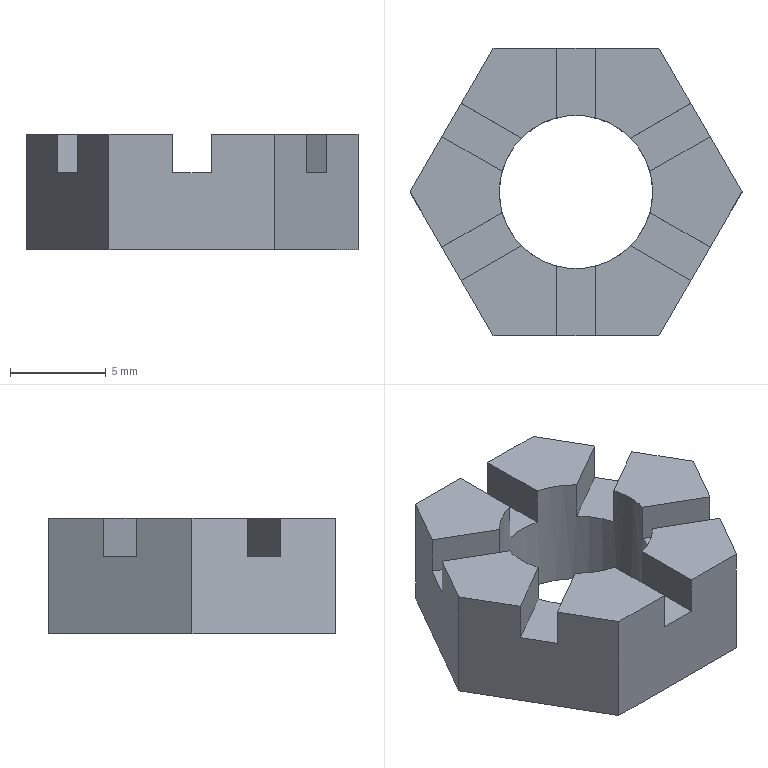Part | SolidWorks | features BaseBody 1 | 1 solid | 33 faces | box 17.321 x 15 x 6 mm | volume 782.532 mm3 | plane 31 | cylinder 2 | commonest cylinder face diameters 8 x2
STEP:
#1=CARTESIAN_POINT('',(4.,0.,6.));
#2=VERTEX_POINT('',#1);
#3=CARTESIAN_POINT('',(3.854,-1.07,6.));
#4=VERTEX_POINT('',#3);
#5=CARTESIAN_POINT('',(0.,0.,6.));
#6=DIRECTION('',(0.,0.,-1.));
#7=DIRECTION('',(-1.,0.,0.));
#8=AXIS2_PLACEMENT_3D('',#5,#6,#7);
#9=CIRCLE('',#8,4.);
#10=EDGE_CURVE('',#2,#4,#9,.T.);
#11=ORIENTED_EDGE('',*,*,#10,.F.);
#12=CARTESIAN_POINT('',(4.,0.,0.));
#13=VERTEX_POINT('',#12);
#14=CARTESIAN_POINT('',(4.,0.,0.));
#15=DIRECTION('',(0.,0.,-1.));
#16=VECTOR('',#15,1000.);
#17=LINE('',#14,#16);
#18=EDGE_CURVE('',#2,#13,#17,.T.);
#19=ORIENTED_EDGE('',*,*,#18,.T.);
#20=CARTESIAN_POINT('',(-4.,0.,0.));
#21=VERTEX_POINT('',#20);
#22=CARTESIAN_POINT('',(0.,0.,0.));
#23=DIRECTION('',(0.,0.,1.));
#24=DIRECTION('',(-1.,0.,0.));
#25=AXIS2_PLACEMENT_3D('',#22,#23,#24);
#26=CIRCLE('',#25,4.);
#27=EDGE_CURVE('',#21,#13,#26,.T.);
#28=ORIENTED_EDGE('',*,*,#27,.F.);
#29=CARTESIAN_POINT('',(-4.,0.,6.));
#30=VERTEX_POINT('',#29);
#31=CARTESIAN_POINT('',(-4.,0.,0.));
#32=DIRECTION('',(0.,0.,-1.));
#33=VECTOR('',#32,1000.);
#34=LINE('',#31,#33);
#35=EDGE_CURVE('',#30,#21,#34,.T.);
#36=ORIENTED_EDGE('',*,*,#35,.F.);
#37=CARTESIAN_POINT('',(-3.854,-1.07,6.));
#38=VERTEX_POINT('',#37);
#39=CARTESIAN_POINT('',(0.,0.,6.));
#40=DIRECTION('',(0.,0.,-1.));
#41=DIRECTION('',(-1.,0.,0.));
#42=AXIS2_PLACEMENT_3D('',#39,#40,#41);
#43=CIRCLE('',#42,4.);
#44=EDGE_CURVE('',#38,#30,#43,.T.);
#45=ORIENTED_EDGE('',*,*,#44,.F.);
#46=CARTESIAN_POINT('',(-3.854,-1.07,4.));
#47=VERTEX_POINT('',#46);
#48=CARTESIAN_POINT('',(-3.854,-1.07,0.));
#49=DIRECTION('',(0.,0.,-1.));
#50=VECTOR('',#49,1000.);
#51=LINE('',#48,#50);
#52=EDGE_CURVE('',#38,#47,#51,.T.);
#53=ORIENTED_EDGE('',*,*,#52,.T.);
#54=CARTESIAN_POINT('',(-2.854,-2.803,4.));
#55=VERTEX_POINT('',#54);
#56=CARTESIAN_POINT('',(0.,0.,4.));
#57=DIRECTION('',(0.,0.,1.));
#58=DIRECTION('',(-1.,0.,0.));
#59=AXIS2_PLACEMENT_3D('',#56,#57,#58);
#60=CIRCLE('',#59,4.);
#61=EDGE_CURVE('',#47,#55,#60,.T.);
#62=ORIENTED_EDGE('',*,*,#61,.T.);
#63=CARTESIAN_POINT('',(-2.854,-2.803,6.));
#64=VERTEX_POINT('',#63);
#65=CARTESIAN_POINT('',(-2.854,-2.803,0.));
#66=DIRECTION('',(0.,0.,1.));
#67=VECTOR('',#66,1000.);
#68=LINE('',#65,#67);
#69=EDGE_CURVE('',#55,#64,#68,.T.);
#70=ORIENTED_EDGE('',*,*,#69,.T.);
#71=CARTESIAN_POINT('',(-1.,-3.873,6.));
#72=VERTEX_POINT('',#71);
#73=CARTESIAN_POINT('',(0.,0.,6.));
#74=DIRECTION('',(0.,0.,-1.));
#75=DIRECTION('',(-1.,0.,0.));
#76=AXIS2_PLACEMENT_3D('',#73,#74,#75);
#77=CIRCLE('',#76,4.);
#78=EDGE_CURVE('',#72,#64,#77,.T.);
#79=ORIENTED_EDGE('',*,*,#78,.F.);
#80=CARTESIAN_POINT('',(-1.,-3.873,4.));
#81=VERTEX_POINT('',#80);
#82=CARTESIAN_POINT('',(-1.,-3.873,0.));
#83=DIRECTION('',(0.,0.,-1.));
#84=VECTOR('',#83,1000.);
#85=LINE('',#82,#84);
#86=EDGE_CURVE('',#72,#81,#85,.T.);
#87=ORIENTED_EDGE('',*,*,#86,.T.);
#88=CARTESIAN_POINT('',(1.,-3.873,4.));
#89=VERTEX_POINT('',#88);
#90=CARTESIAN_POINT('',(0.,0.,4.));
#91=DIRECTION('',(0.,0.,1.));
#92=DIRECTION('',(-1.,0.,0.));
#93=AXIS2_PLACEMENT_3D('',#90,#91,#92);
#94=CIRCLE('',#93,4.);
#95=EDGE_CURVE('',#81,#89,#94,.T.);
#96=ORIENTED_EDGE('',*,*,#95,.T.);
#97=CARTESIAN_POINT('',(1.,-3.873,6.));
#98=VERTEX_POINT('',#97);
#99=CARTESIAN_POINT('',(1.,-3.873,0.));
#100=DIRECTION('',(0.,0.,1.));
#101=VECTOR('',#100,1000.);
#102=LINE('',#99,#101);
#103=EDGE_CURVE('',#89,#98,#102,.T.);
#104=ORIENTED_EDGE('',*,*,#103,.T.);
#105=CARTESIAN_POINT('',(2.854,-2.803,6.));
#106=VERTEX_POINT('',#105);
#107=CARTESIAN_POINT('',(0.,0.,6.));
#108=DIRECTION('',(0.,0.,-1.));
#109=DIRECTION('',(-1.,0.,0.));
#110=AXIS2_PLACEMENT_3D('',#107,#108,#109);
#111=CIRCLE('',#110,4.);
#112=EDGE_CURVE('',#106,#98,#111,.T.);
#113=ORIENTED_EDGE('',*,*,#112,.F.);
#114=CARTESIAN_POINT('',(2.854,-2.803,4.));
#115=VERTEX_POINT('',#114);
#116=CARTESIAN_POINT('',(2.854,-2.803,0.));
#117=DIRECTION('',(0.,0.,-1.));
#118=VECTOR('',#117,1000.);
#119=LINE('',#116,#118);
#120=EDGE_CURVE('',#106,#115,#119,.T.);
#121=ORIENTED_EDGE('',*,*,#120,.T.);
#122=CARTESIAN_POINT('',(3.854,-1.07,4.));
#123=VERTEX_POINT('',#122);
#124=CARTESIAN_POINT('',(0.,0.,4.));
#125=DIRECTION('',(0.,0.,1.));
#126=DIRECTION('',(-1.,0.,0.));
#127=AXIS2_PLACEMENT_3D('',#124,#125,#126);
#128=CIRCLE('',#127,4.);
#129=EDGE_CURVE('',#115,#123,#128,.T.);
#130=ORIENTED_EDGE('',*,*,#129,.T.);
#131=CARTESIAN_POINT('',(3.854,-1.07,0.));
#132=DIRECTION('',(0.,0.,1.));
#133=VECTOR('',#132,1000.);
#134=LINE('',#131,#133);
#135=EDGE_CURVE('',#123,#4,#134,.T.);
#136=ORIENTED_EDGE('',*,*,#135,.T.);
#137=EDGE_LOOP('',(#11,#19,#28,#36,#45,#53,#62,#70,#79,#87,#96,#104,#113,#121,#130,#136));
#138=FACE_OUTER_BOUND('',#137,.T.);
#139=CARTESIAN_POINT('',(0.,0.,0.));
#140=DIRECTION('',(0.,0.,-1.));
#141=DIRECTION('',(-1.,0.,0.));
#142=AXIS2_PLACEMENT_3D('',#139,#140,#141);
#143=CYLINDRICAL_SURFACE('',#142,4.);
#144=ADVANCED_FACE('',(#138),#143,.F.);
#145=CARTESIAN_POINT('',(-3.854,1.07,4.));
#146=VERTEX_POINT('',#145);
#147=CARTESIAN_POINT('',(-3.854,1.07,6.));
#148=VERTEX_POINT('',#147);
#149=CARTESIAN_POINT('',(-3.854,1.07,0.));
#150=DIRECTION('',(0.,0.,1.));
#151=VECTOR('',#150,1000.);
#152=LINE('',#149,#151);
#153=EDGE_CURVE('',#146,#148,#152,.T.);
#154=ORIENTED_EDGE('',*,*,#153,.F.);
#155=CARTESIAN_POINT('',(-6.995,2.884,4.));
#156=VERTEX_POINT('',#155);
#157=CARTESIAN_POINT('',(5.995,-4.616,4.));
#158=DIRECTION('',(-0.866,0.5,0.));
#159=VECTOR('',#158,1000.);
#160=LINE('',#157,#159);
#161=EDGE_CURVE('',#146,#156,#160,.T.);
#162=ORIENTED_EDGE('',*,*,#161,.T.);
#163=CARTESIAN_POINT('',(-6.995,2.884,6.));
#164=VERTEX_POINT('',#163);
#165=CARTESIAN_POINT('',(-6.995,2.884,3.));
#166=DIRECTION('',(0.,0.,-1.));
#167=VECTOR('',#166,1000.);
#168=LINE('',#165,#167);
#169=EDGE_CURVE('',#164,#156,#168,.T.);
#170=ORIENTED_EDGE('',*,*,#169,.F.);
#171=CARTESIAN_POINT('',(2.748,-2.741,6.));
#172=DIRECTION('',(-0.866,0.5,0.));
#173=VECTOR('',#172,1000.);
#174=LINE('',#171,#173);
#175=EDGE_CURVE('',#148,#164,#174,.T.);
#176=ORIENTED_EDGE('',*,*,#175,.F.);
#177=EDGE_LOOP('',(#154,#162,#170,#176));
#178=FACE_OUTER_BOUND('',#177,.T.);
#179=CARTESIAN_POINT('',(5.995,-4.616,6.));
#180=DIRECTION('',(-0.5,-0.866,0.));
#181=DIRECTION('',(-0.866,0.5,0.));
#182=AXIS2_PLACEMENT_3D('',#179,#180,#181);
#183=PLANE('',#182);
#184=ADVANCED_FACE('',(#178),#183,.F.);
#185=ORIENTED_EDGE('',*,*,#135,.F.);
#186=CARTESIAN_POINT('',(6.995,-2.884,4.));
#187=VERTEX_POINT('',#186);
#188=CARTESIAN_POINT('',(-5.995,4.616,4.));
#189=DIRECTION('',(0.866,-0.5,0.));
#190=VECTOR('',#189,1000.);
#191=LINE('',#188,#190);
#192=EDGE_CURVE('',#123,#187,#191,.T.);
#193=ORIENTED_EDGE('',*,*,#192,.T.);
#194=CARTESIAN_POINT('',(6.995,-2.884,6.));
#195=VERTEX_POINT('',#194);
#196=CARTESIAN_POINT('',(6.995,-2.884,3.));
#197=DIRECTION('',(0.,0.,-1.));
#198=VECTOR('',#197,1000.);
#199=LINE('',#196,#198);
#200=EDGE_CURVE('',#195,#187,#199,.T.);
#201=ORIENTED_EDGE('',*,*,#200,.F.);
#202=CARTESIAN_POINT('',(-2.748,2.741,6.));
#203=DIRECTION('',(0.866,-0.5,0.));
#204=VECTOR('',#203,1000.);
#205=LINE('',#202,#204);
#206=EDGE_CURVE('',#4,#195,#205,.T.);
#207=ORIENTED_EDGE('',*,*,#206,.F.);
#208=EDGE_LOOP('',(#185,#193,#201,#207));
#209=FACE_OUTER_BOUND('',#208,.T.);
#210=CARTESIAN_POINT('',(-5.995,4.616,6.));
#211=DIRECTION('',(0.5,0.866,0.));
#212=DIRECTION('',(0.,0.,-1.));
#213=AXIS2_PLACEMENT_3D('',#210,#211,#212);
#214=PLANE('',#213);
#215=ADVANCED_FACE('',(#209),#214,.F.);
#216=ORIENTED_EDGE('',*,*,#69,.F.);
#217=CARTESIAN_POINT('',(-5.995,-4.616,4.));
#218=VERTEX_POINT('',#217);
#219=CARTESIAN_POINT('',(6.995,2.884,4.));
#220=DIRECTION('',(-0.866,-0.5,0.));
#221=VECTOR('',#220,1000.);
#222=LINE('',#219,#221);
#223=EDGE_CURVE('',#55,#218,#222,.T.);
#224=ORIENTED_EDGE('',*,*,#223,.T.);
#225=CARTESIAN_POINT('',(-5.995,-4.616,6.));
#226=VERTEX_POINT('',#225);
#227=CARTESIAN_POINT('',(-5.995,-4.616,3.));
#228=DIRECTION('',(0.,0.,-1.));
#229=VECTOR('',#228,1000.);
#230=LINE('',#227,#229);
#231=EDGE_CURVE('',#226,#218,#230,.T.);
#232=ORIENTED_EDGE('',*,*,#231,.F.);
#233=CARTESIAN_POINT('',(3.748,1.009,6.));
#234=DIRECTION('',(-0.866,-0.5,0.));
#235=VECTOR('',#234,1000.);
#236=LINE('',#233,#235);
#237=EDGE_CURVE('',#64,#226,#236,.T.);
#238=ORIENTED_EDGE('',*,*,#237,.F.);
#239=EDGE_LOOP('',(#216,#224,#232,#238));
#240=FACE_OUTER_BOUND('',#239,.T.);
#241=CARTESIAN_POINT('',(6.995,2.884,6.));
#242=DIRECTION('',(0.5,-0.866,0.));
#243=DIRECTION('',(0.,0.,-1.));
#244=AXIS2_PLACEMENT_3D('',#241,#242,#243);
#245=PLANE('',#244);
#246=ADVANCED_FACE('',(#240),#245,.F.);
#247=ORIENTED_EDGE('',*,*,#61,.F.);
#248=CARTESIAN_POINT('',(-6.995,-2.884,4.));
#249=VERTEX_POINT('',#248);
#250=CARTESIAN_POINT('',(-6.995,-2.884,4.));
#251=DIRECTION('',(0.866,0.5,0.));
#252=VECTOR('',#251,1000.);
#253=LINE('',#250,#252);
#254=EDGE_CURVE('',#249,#47,#253,.T.);
#255=ORIENTED_EDGE('',*,*,#254,.F.);
#256=CARTESIAN_POINT('',(-7.578,-1.875,4.));
#257=DIRECTION('',(-0.5,0.866,0.));
#258=VECTOR('',#257,1000.);
#259=LINE('',#256,#258);
#260=EDGE_CURVE('',#218,#249,#259,.T.);
#261=ORIENTED_EDGE('',*,*,#260,.F.);
#262=ORIENTED_EDGE('',*,*,#223,.F.);
#263=EDGE_LOOP('',(#247,#255,#261,#262));
#264=FACE_OUTER_BOUND('',#263,.T.);
#265=CARTESIAN_POINT('',(0.,0.,4.));
#266=DIRECTION('',(0.,0.,-1.));
#267=DIRECTION('',(0.,-1.,0.));
#268=AXIS2_PLACEMENT_3D('',#265,#266,#267);
#269=PLANE('',#268);
#270=ADVANCED_FACE('',(#264),#269,.F.);
#271=ORIENTED_EDGE('',*,*,#129,.F.);
#272=CARTESIAN_POINT('',(5.995,-4.616,4.));
#273=VERTEX_POINT('',#272);
#274=CARTESIAN_POINT('',(5.995,-4.616,4.));
#275=DIRECTION('',(-0.866,0.5,0.));
#276=VECTOR('',#275,1000.);
#277=LINE('',#274,#276);
#278=EDGE_CURVE('',#273,#115,#277,.T.);
#279=ORIENTED_EDGE('',*,*,#278,.F.);
#280=CARTESIAN_POINT('',(5.413,-5.625,4.));
#281=DIRECTION('',(-0.5,-0.866,0.));
#282=VECTOR('',#281,1000.);
#283=LINE('',#280,#282);
#284=EDGE_CURVE('',#187,#273,#283,.T.);
#285=ORIENTED_EDGE('',*,*,#284,.F.);
#286=ORIENTED_EDGE('',*,*,#192,.F.);
#287=EDGE_LOOP('',(#271,#279,#285,#286));
#288=FACE_OUTER_BOUND('',#287,.T.);
#289=CARTESIAN_POINT('',(0.,0.,4.));
#290=DIRECTION('',(0.,0.,-1.));
#291=DIRECTION('',(0.,-1.,0.));
#292=AXIS2_PLACEMENT_3D('',#289,#290,#291);
#293=PLANE('',#292);
#294=ADVANCED_FACE('',(#288),#293,.F.);
#295=CARTESIAN_POINT('',(3.854,1.07,4.));
#296=VERTEX_POINT('',#295);
#297=CARTESIAN_POINT('',(2.854,2.803,4.));
#298=VERTEX_POINT('',#297);
#299=CARTESIAN_POINT('',(0.,0.,4.));
#300=DIRECTION('',(0.,0.,1.));
#301=DIRECTION('',(-1.,0.,0.));
#302=AXIS2_PLACEMENT_3D('',#299,#300,#301);
#303=CIRCLE('',#302,4.);
#304=EDGE_CURVE('',#296,#298,#303,.T.);
#305=ORIENTED_EDGE('',*,*,#304,.F.);
#306=CARTESIAN_POINT('',(6.995,2.884,4.));
#307=VERTEX_POINT('',#306);
#308=CARTESIAN_POINT('',(6.995,2.884,4.));
#309=DIRECTION('',(-0.866,-0.5,0.));
#310=VECTOR('',#309,1000.);
#311=LINE('',#308,#310);
#312=EDGE_CURVE('',#307,#296,#311,.T.);
#313=ORIENTED_EDGE('',*,*,#312,.F.);
#314=CARTESIAN_POINT('',(5.995,4.616,4.));
#315=VERTEX_POINT('',#314);
#316=CARTESIAN_POINT('',(7.578,1.875,4.));
#317=DIRECTION('',(0.5,-0.866,0.));
#318=VECTOR('',#317,1000.);
#319=LINE('',#316,#318);
#320=EDGE_CURVE('',#315,#307,#319,.T.);
#321=ORIENTED_EDGE('',*,*,#320,.F.);
#322=CARTESIAN_POINT('',(-6.995,-2.884,4.));
#323=DIRECTION('',(0.866,0.5,0.));
#324=VECTOR('',#323,1000.);
#325=LINE('',#322,#324);
#326=EDGE_CURVE('',#298,#315,#325,.T.);
#327=ORIENTED_EDGE('',*,*,#326,.F.);
#328=EDGE_LOOP('',(#305,#313,#321,#327));
#329=FACE_OUTER_BOUND('',#328,.T.);
#330=CARTESIAN_POINT('',(0.,0.,4.));
#331=DIRECTION('',(0.,0.,-1.));
#332=DIRECTION('',(0.,-1.,0.));
#333=AXIS2_PLACEMENT_3D('',#330,#331,#332);
#334=PLANE('',#333);
#335=ADVANCED_FACE('',(#329),#334,.F.);
#336=CARTESIAN_POINT('',(-2.854,2.803,4.));
#337=VERTEX_POINT('',#336);
#338=CARTESIAN_POINT('',(0.,0.,4.));
#339=DIRECTION('',(0.,0.,1.));
#340=DIRECTION('',(-1.,0.,0.));
#341=AXIS2_PLACEMENT_3D('',#338,#339,#340);
#342=CIRCLE('',#341,4.);
#343=EDGE_CURVE('',#337,#146,#342,.T.);
#344=ORIENTED_EDGE('',*,*,#343,.F.);
#345=CARTESIAN_POINT('',(-5.995,4.616,4.));
#346=VERTEX_POINT('',#345);
#347=CARTESIAN_POINT('',(-5.995,4.616,4.));
#348=DIRECTION('',(0.866,-0.5,0.));
#349=VECTOR('',#348,1000.);
#350=LINE('',#347,#349);
#351=EDGE_CURVE('',#346,#337,#350,.T.);
#352=ORIENTED_EDGE('',*,*,#351,.F.);
#353=CARTESIAN_POINT('',(-5.413,5.625,4.));
#354=DIRECTION('',(0.5,0.866,0.));
#355=VECTOR('',#354,1000.);
#356=LINE('',#353,#355);
#357=EDGE_CURVE('',#156,#346,#356,.T.);
#358=ORIENTED_EDGE('',*,*,#357,.F.);
#359=ORIENTED_EDGE('',*,*,#161,.F.);
#360=EDGE_LOOP('',(#344,#352,#358,#359));
#361=FACE_OUTER_BOUND('',#360,.T.);
#362=CARTESIAN_POINT('',(0.,0.,4.));
#363=DIRECTION('',(0.,0.,-1.));
#364=DIRECTION('',(0.,-1.,0.));
#365=AXIS2_PLACEMENT_3D('',#362,#363,#364);
#366=PLANE('',#365);
#367=ADVANCED_FACE('',(#361),#366,.F.);
#368=CARTESIAN_POINT('',(2.854,2.803,6.));
#369=VERTEX_POINT('',#368);
#370=CARTESIAN_POINT('',(2.854,2.803,0.));
#371=DIRECTION('',(0.,0.,1.));
#372=VECTOR('',#371,1000.);
#373=LINE('',#370,#372);
#374=EDGE_CURVE('',#298,#369,#373,.T.);
#375=ORIENTED_EDGE('',*,*,#374,.F.);
#376=ORIENTED_EDGE('',*,*,#326,.T.);
#377=CARTESIAN_POINT('',(5.995,4.616,6.));
#378=VERTEX_POINT('',#377);
#379=CARTESIAN_POINT('',(5.995,4.616,3.));
#380=DIRECTION('',(0.,0.,-1.));
#381=VECTOR('',#380,1000.);
#382=LINE('',#379,#381);
#383=EDGE_CURVE('',#378,#315,#382,.T.);
#384=ORIENTED_EDGE('',*,*,#383,.F.);
#385=CARTESIAN_POINT('',(-3.748,-1.009,6.));
#386=DIRECTION('',(0.866,0.5,0.));
#387=VECTOR('',#386,1000.);
#388=LINE('',#385,#387);
#389=EDGE_CURVE('',#369,#378,#388,.T.);
#390=ORIENTED_EDGE('',*,*,#389,.F.);
#391=EDGE_LOOP('',(#375,#376,#384,#390));
#392=FACE_OUTER_BOUND('',#391,.T.);
#393=CARTESIAN_POINT('',(-6.995,-2.884,6.));
#394=DIRECTION('',(-0.5,0.866,0.));
#395=DIRECTION('',(0.,0.,1.));
#396=AXIS2_PLACEMENT_3D('',#393,#394,#395);
#397=PLANE('',#396);
#398=ADVANCED_FACE('',(#392),#397,.F.);
#399=CARTESIAN_POINT('',(-2.854,2.803,6.));
#400=VERTEX_POINT('',#399);
#401=CARTESIAN_POINT('',(-2.854,2.803,0.));
#402=DIRECTION('',(0.,0.,-1.));
#403=VECTOR('',#402,1000.);
#404=LINE('',#401,#403);
#405=EDGE_CURVE('',#400,#337,#404,.T.);
#406=ORIENTED_EDGE('',*,*,#405,.F.);
#407=CARTESIAN_POINT('',(-5.995,4.616,6.));
#408=VERTEX_POINT('',#407);
#409=CARTESIAN_POINT('',(-2.748,2.741,6.));
#410=DIRECTION('',(0.866,-0.5,0.));
#411=VECTOR('',#410,1000.);
#412=LINE('',#409,#411);
#413=EDGE_CURVE('',#408,#400,#412,.T.);
#414=ORIENTED_EDGE('',*,*,#413,.F.);
#415=CARTESIAN_POINT('',(-5.995,4.616,3.));
#416=DIRECTION('',(0.,0.,1.));
#417=VECTOR('',#416,1000.);
#418=LINE('',#415,#417);
#419=EDGE_CURVE('',#346,#408,#418,.T.);
#420=ORIENTED_EDGE('',*,*,#419,.F.);
#421=ORIENTED_EDGE('',*,*,#351,.T.);
#422=EDGE_LOOP('',(#406,#414,#420,#421));
#423=FACE_OUTER_BOUND('',#422,.T.);
#424=CARTESIAN_POINT('',(-5.995,4.616,6.));
#425=DIRECTION('',(0.5,0.866,0.));
#426=DIRECTION('',(0.,0.,-1.));
#427=AXIS2_PLACEMENT_3D('',#424,#425,#426);
#428=PLANE('',#427);
#429=ADVANCED_FACE('',(#423),#428,.F.);
#430=ORIENTED_EDGE('',*,*,#120,.F.);
#431=CARTESIAN_POINT('',(5.995,-4.616,6.));
#432=VERTEX_POINT('',#431);
#433=CARTESIAN_POINT('',(2.748,-2.741,6.));
#434=DIRECTION('',(-0.866,0.5,0.));
#435=VECTOR('',#434,1000.);
#436=LINE('',#433,#435);
#437=EDGE_CURVE('',#432,#106,#436,.T.);
#438=ORIENTED_EDGE('',*,*,#437,.F.);
#439=CARTESIAN_POINT('',(5.995,-4.616,3.));
#440=DIRECTION('',(0.,0.,1.));
#441=VECTOR('',#440,1000.);
#442=LINE('',#439,#441);
#443=EDGE_CURVE('',#273,#432,#442,.T.);
#444=ORIENTED_EDGE('',*,*,#443,.F.);
#445=ORIENTED_EDGE('',*,*,#278,.T.);
#446=EDGE_LOOP('',(#430,#438,#444,#445));
#447=FACE_OUTER_BOUND('',#446,.T.);
#448=CARTESIAN_POINT('',(5.995,-4.616,6.));
#449=DIRECTION('',(-0.5,-0.866,0.));
#450=DIRECTION('',(-0.866,0.5,0.));
#451=AXIS2_PLACEMENT_3D('',#448,#449,#450);
#452=PLANE('',#451);
#453=ADVANCED_FACE('',(#447),#452,.F.);
#454=ORIENTED_EDGE('',*,*,#52,.F.);
#455=CARTESIAN_POINT('',(-6.995,-2.884,6.));
#456=VERTEX_POINT('',#455);
#457=CARTESIAN_POINT('',(-3.748,-1.009,6.));
#458=DIRECTION('',(0.866,0.5,0.));
#459=VECTOR('',#458,1000.);
#460=LINE('',#457,#459);
#461=EDGE_CURVE('',#456,#38,#460,.T.);
#462=ORIENTED_EDGE('',*,*,#461,.F.);
#463=CARTESIAN_POINT('',(-6.995,-2.884,3.));
#464=DIRECTION('',(0.,0.,1.));
#465=VECTOR('',#464,1000.);
#466=LINE('',#463,#465);
#467=EDGE_CURVE('',#249,#456,#466,.T.);
#468=ORIENTED_EDGE('',*,*,#467,.F.);
#469=ORIENTED_EDGE('',*,*,#254,.T.);
#470=EDGE_LOOP('',(#454,#462,#468,#469));
#471=FACE_OUTER_BOUND('',#470,.T.);
#472=CARTESIAN_POINT('',(-6.995,-2.884,6.));
#473=DIRECTION('',(-0.5,0.866,0.));
#474=DIRECTION('',(0.,0.,1.));
#475=AXIS2_PLACEMENT_3D('',#472,#473,#474);
#476=PLANE('',#475);
#477=ADVANCED_FACE('',(#471),#476,.F.);
#478=CARTESIAN_POINT('',(3.854,1.07,6.));
#479=VERTEX_POINT('',#478);
#480=CARTESIAN_POINT('',(3.854,1.07,0.));
#481=DIRECTION('',(0.,0.,-1.));
#482=VECTOR('',#481,1000.);
#483=LINE('',#480,#482);
#484=EDGE_CURVE('',#479,#296,#483,.T.);
#485=ORIENTED_EDGE('',*,*,#484,.F.);
#486=CARTESIAN_POINT('',(6.995,2.884,6.));
#487=VERTEX_POINT('',#486);
#488=CARTESIAN_POINT('',(3.748,1.009,6.));
#489=DIRECTION('',(-0.866,-0.5,0.));
#490=VECTOR('',#489,1000.);
#491=LINE('',#488,#490);
#492=EDGE_CURVE('',#487,#479,#491,.T.);
#493=ORIENTED_EDGE('',*,*,#492,.F.);
#494=CARTESIAN_POINT('',(6.995,2.884,3.));
#495=DIRECTION('',(0.,0.,1.));
#496=VECTOR('',#495,1000.);
#497=LINE('',#494,#496);
#498=EDGE_CURVE('',#307,#487,#497,.T.);
#499=ORIENTED_EDGE('',*,*,#498,.F.);
#500=ORIENTED_EDGE('',*,*,#312,.T.);
#501=EDGE_LOOP('',(#485,#493,#499,#500));
#502=FACE_OUTER_BOUND('',#501,.T.);
#503=CARTESIAN_POINT('',(6.995,2.884,6.));
#504=DIRECTION('',(0.5,-0.866,0.));
#505=DIRECTION('',(0.,0.,-1.));
#506=AXIS2_PLACEMENT_3D('',#503,#504,#505);
#507=PLANE('',#506);
#508=ADVANCED_FACE('',(#502),#507,.F.);
#509=ORIENTED_EDGE('',*,*,#200,.T.);
#510=ORIENTED_EDGE('',*,*,#284,.T.);
#511=ORIENTED_EDGE('',*,*,#443,.T.);
#512=CARTESIAN_POINT('',(4.33,-7.5,6.));
#513=VERTEX_POINT('',#512);
#514=CARTESIAN_POINT('',(8.66,0.,6.));
#515=DIRECTION('',(0.5,0.866,0.));
#516=VECTOR('',#515,1000.);
#517=LINE('',#514,#516);
#518=EDGE_CURVE('',#513,#432,#517,.T.);
#519=ORIENTED_EDGE('',*,*,#518,.F.);
#520=CARTESIAN_POINT('',(4.33,-7.5,0.));
#521=VERTEX_POINT('',#520);
#522=CARTESIAN_POINT('',(4.33,-7.5,0.));
#523=DIRECTION('',(0.,0.,1.));
#524=VECTOR('',#523,1000.);
#525=LINE('',#522,#524);
#526=EDGE_CURVE('',#521,#513,#525,.T.);
#527=ORIENTED_EDGE('',*,*,#526,.F.);
#528=CARTESIAN_POINT('',(8.66,0.,0.));
#529=VERTEX_POINT('',#528);
#530=CARTESIAN_POINT('',(8.66,0.,0.));
#531=DIRECTION('',(-0.5,-0.866,0.));
#532=VECTOR('',#531,1000.);
#533=LINE('',#530,#532);
#534=EDGE_CURVE('',#529,#521,#533,.T.);
#535=ORIENTED_EDGE('',*,*,#534,.F.);
#536=CARTESIAN_POINT('',(8.66,0.,6.));
#537=VERTEX_POINT('',#536);
#538=CARTESIAN_POINT('',(8.66,0.,0.));
#539=DIRECTION('',(0.,0.,1.));
#540=VECTOR('',#539,1000.);
#541=LINE('',#538,#540);
#542=EDGE_CURVE('',#529,#537,#541,.T.);
#543=ORIENTED_EDGE('',*,*,#542,.T.);
#544=CARTESIAN_POINT('',(8.66,0.,6.));
#545=DIRECTION('',(0.5,0.866,0.));
#546=VECTOR('',#545,1000.);
#547=LINE('',#544,#546);
#548=EDGE_CURVE('',#195,#537,#547,.T.);
#549=ORIENTED_EDGE('',*,*,#548,.F.);
#550=EDGE_LOOP('',(#509,#510,#511,#519,#527,#535,#543,#549));
#551=FACE_OUTER_BOUND('',#550,.T.);
#552=CARTESIAN_POINT('',(4.33,-7.5,0.));
#553=DIRECTION('',(0.866,-0.5,0.));
#554=DIRECTION('',(0.,0.,-1.));
#555=AXIS2_PLACEMENT_3D('',#552,#553,#554);
#556=PLANE('',#555);
#557=ADVANCED_FACE('',(#551),#556,.T.);
#558=ORIENTED_EDGE('',*,*,#231,.T.);
#559=ORIENTED_EDGE('',*,*,#260,.T.);
#560=ORIENTED_EDGE('',*,*,#467,.T.);
#561=CARTESIAN_POINT('',(-8.66,0.,6.));
#562=VERTEX_POINT('',#561);
#563=CARTESIAN_POINT('',(-4.33,-7.5,6.));
#564=DIRECTION('',(0.5,-0.866,0.));
#565=VECTOR('',#564,1000.);
#566=LINE('',#563,#565);
#567=EDGE_CURVE('',#562,#456,#566,.T.);
#568=ORIENTED_EDGE('',*,*,#567,.F.);
#569=CARTESIAN_POINT('',(-8.66,0.,0.));
#570=VERTEX_POINT('',#569);
#571=CARTESIAN_POINT('',(-8.66,0.,0.));
#572=DIRECTION('',(0.,0.,1.));
#573=VECTOR('',#572,1000.);
#574=LINE('',#571,#573);
#575=EDGE_CURVE('',#570,#562,#574,.T.);
#576=ORIENTED_EDGE('',*,*,#575,.F.);
#577=CARTESIAN_POINT('',(-4.33,-7.5,0.));
#578=VERTEX_POINT('',#577);
#579=CARTESIAN_POINT('',(-4.33,-7.5,0.));
#580=DIRECTION('',(-0.5,0.866,0.));
#581=VECTOR('',#580,1000.);
#582=LINE('',#579,#581);
#583=EDGE_CURVE('',#578,#570,#582,.T.);
#584=ORIENTED_EDGE('',*,*,#583,.F.);
#585=CARTESIAN_POINT('',(-4.33,-7.5,6.));
#586=VERTEX_POINT('',#585);
#587=CARTESIAN_POINT('',(-4.33,-7.5,0.));
#588=DIRECTION('',(0.,0.,1.));
#589=VECTOR('',#588,1000.);
#590=LINE('',#587,#589);
#591=EDGE_CURVE('',#578,#586,#590,.T.);
#592=ORIENTED_EDGE('',*,*,#591,.T.);
#593=CARTESIAN_POINT('',(-4.33,-7.5,6.));
#594=DIRECTION('',(0.5,-0.866,0.));
#595=VECTOR('',#594,1000.);
#596=LINE('',#593,#595);
#597=EDGE_CURVE('',#226,#586,#596,.T.);
#598=ORIENTED_EDGE('',*,*,#597,.F.);
#599=EDGE_LOOP('',(#558,#559,#560,#568,#576,#584,#592,#598));
#600=FACE_OUTER_BOUND('',#599,.T.);
#601=CARTESIAN_POINT('',(-8.66,0.,0.));
#602=DIRECTION('',(-0.866,-0.5,0.));
#603=DIRECTION('',(-0.5,0.866,0.));
#604=AXIS2_PLACEMENT_3D('',#601,#602,#603);
#605=PLANE('',#604);
#606=ADVANCED_FACE('',(#600),#605,.T.);
#607=ORIENTED_EDGE('',*,*,#237,.T.);
#608=ORIENTED_EDGE('',*,*,#597,.T.);
#609=CARTESIAN_POINT('',(-1.,-7.5,6.));
#610=VERTEX_POINT('',#609);
#611=CARTESIAN_POINT('',(4.33,-7.5,6.));
#612=DIRECTION('',(1.,0.,0.));
#613=VECTOR('',#612,1000.);
#614=LINE('',#611,#613);
#615=EDGE_CURVE('',#586,#610,#614,.T.);
#616=ORIENTED_EDGE('',*,*,#615,.T.);
#617=CARTESIAN_POINT('',(-1.,-3.75,6.));
#618=DIRECTION('',(0.,1.,0.));
#619=VECTOR('',#618,1000.);
#620=LINE('',#617,#619);
#621=EDGE_CURVE('',#610,#72,#620,.T.);
#622=ORIENTED_EDGE('',*,*,#621,.T.);
#623=ORIENTED_EDGE('',*,*,#78,.T.);
#624=EDGE_LOOP('',(#607,#608,#616,#622,#623));
#625=FACE_OUTER_BOUND('',#624,.T.);
#626=CARTESIAN_POINT('',(0.,0.,6.));
#627=DIRECTION('',(0.,0.,1.));
#628=DIRECTION('',(1.,0.,0.));
#629=AXIS2_PLACEMENT_3D('',#626,#627,#628);
#630=PLANE('',#629);
#631=ADVANCED_FACE('',(#625),#630,.T.);
#632=ORIENTED_EDGE('',*,*,#175,.T.);
#633=CARTESIAN_POINT('',(-8.66,0.,6.));
#634=DIRECTION('',(-0.5,-0.866,0.));
#635=VECTOR('',#634,1000.);
#636=LINE('',#633,#635);
#637=EDGE_CURVE('',#164,#562,#636,.T.);
#638=ORIENTED_EDGE('',*,*,#637,.T.);
#639=ORIENTED_EDGE('',*,*,#567,.T.);
#640=ORIENTED_EDGE('',*,*,#461,.T.);
#641=ORIENTED_EDGE('',*,*,#44,.T.);
#642=CARTESIAN_POINT('',(0.,0.,6.));
#643=DIRECTION('',(0.,0.,-1.));
#644=DIRECTION('',(-1.,0.,0.));
#645=AXIS2_PLACEMENT_3D('',#642,#643,#644);
#646=CIRCLE('',#645,4.);
#647=EDGE_CURVE('',#30,#148,#646,.T.);
#648=ORIENTED_EDGE('',*,*,#647,.T.);
#649=EDGE_LOOP('',(#632,#638,#639,#640,#641,#648));
#650=FACE_OUTER_BOUND('',#649,.T.);
#651=CARTESIAN_POINT('',(0.,0.,6.));
#652=DIRECTION('',(0.,0.,1.));
#653=DIRECTION('',(1.,0.,0.));
#654=AXIS2_PLACEMENT_3D('',#651,#652,#653);
#655=PLANE('',#654);
#656=ADVANCED_FACE('',(#650),#655,.T.);
#657=ORIENTED_EDGE('',*,*,#383,.T.);
#658=ORIENTED_EDGE('',*,*,#320,.T.);
#659=ORIENTED_EDGE('',*,*,#498,.T.);
#660=CARTESIAN_POINT('',(4.33,7.5,6.));
#661=DIRECTION('',(-0.5,0.866,0.));
#662=VECTOR('',#661,1000.);
#663=LINE('',#660,#662);
#664=EDGE_CURVE('',#537,#487,#663,.T.);
#665=ORIENTED_EDGE('',*,*,#664,.F.);
#666=ORIENTED_EDGE('',*,*,#542,.F.);
#667=CARTESIAN_POINT('',(4.33,7.5,0.));
#668=VERTEX_POINT('',#667);
#669=CARTESIAN_POINT('',(4.33,7.5,0.));
#670=DIRECTION('',(0.5,-0.866,0.));
#671=VECTOR('',#670,1000.);
#672=LINE('',#669,#671);
#673=EDGE_CURVE('',#668,#529,#672,.T.);
#674=ORIENTED_EDGE('',*,*,#673,.F.);
#675=CARTESIAN_POINT('',(4.33,7.5,6.));
#676=VERTEX_POINT('',#675);
#677=CARTESIAN_POINT('',(4.33,7.5,0.));
#678=DIRECTION('',(0.,0.,1.));
#679=VECTOR('',#678,1000.);
#680=LINE('',#677,#679);
#681=EDGE_CURVE('',#668,#676,#680,.T.);
#682=ORIENTED_EDGE('',*,*,#681,.T.);
#683=CARTESIAN_POINT('',(4.33,7.5,6.));
#684=DIRECTION('',(-0.5,0.866,0.));
#685=VECTOR('',#684,1000.);
#686=LINE('',#683,#685);
#687=EDGE_CURVE('',#378,#676,#686,.T.);
#688=ORIENTED_EDGE('',*,*,#687,.F.);
#689=EDGE_LOOP('',(#657,#658,#659,#665,#666,#674,#682,#688));
#690=FACE_OUTER_BOUND('',#689,.T.);
#691=CARTESIAN_POINT('',(8.66,0.,0.));
#692=DIRECTION('',(0.866,0.5,0.));
#693=DIRECTION('',(0.,0.,-1.));
#694=AXIS2_PLACEMENT_3D('',#691,#692,#693);
#695=PLANE('',#694);
#696=ADVANCED_FACE('',(#690),#695,.T.);
#697=ORIENTED_EDGE('',*,*,#389,.T.);
#698=ORIENTED_EDGE('',*,*,#687,.T.);
#699=CARTESIAN_POINT('',(1.,7.5,6.));
#700=VERTEX_POINT('',#699);
#701=CARTESIAN_POINT('',(-4.33,7.5,6.));
#702=DIRECTION('',(-1.,0.,0.));
#703=VECTOR('',#702,1000.);
#704=LINE('',#701,#703);
#705=EDGE_CURVE('',#676,#700,#704,.T.);
#706=ORIENTED_EDGE('',*,*,#705,.T.);
#707=CARTESIAN_POINT('',(1.,3.873,6.));
#708=VERTEX_POINT('',#707);
#709=CARTESIAN_POINT('',(1.,3.75,6.));
#710=DIRECTION('',(0.,-1.,0.));
#711=VECTOR('',#710,1000.);
#712=LINE('',#709,#711);
#713=EDGE_CURVE('',#700,#708,#712,.T.);
#714=ORIENTED_EDGE('',*,*,#713,.T.);
#715=CARTESIAN_POINT('',(0.,0.,6.));
#716=DIRECTION('',(0.,0.,-1.));
#717=DIRECTION('',(-1.,0.,0.));
#718=AXIS2_PLACEMENT_3D('',#715,#716,#717);
#719=CIRCLE('',#718,4.);
#720=EDGE_CURVE('',#708,#369,#719,.T.);
#721=ORIENTED_EDGE('',*,*,#720,.T.);
#722=EDGE_LOOP('',(#697,#698,#706,#714,#721));
#723=FACE_OUTER_BOUND('',#722,.T.);
#724=CARTESIAN_POINT('',(0.,0.,6.));
#725=DIRECTION('',(0.,0.,1.));
#726=DIRECTION('',(1.,0.,0.));
#727=AXIS2_PLACEMENT_3D('',#724,#725,#726);
#728=PLANE('',#727);
#729=ADVANCED_FACE('',(#723),#728,.T.);
#730=ORIENTED_EDGE('',*,*,#437,.T.);
#731=ORIENTED_EDGE('',*,*,#112,.T.);
#732=CARTESIAN_POINT('',(1.,-7.5,6.));
#733=VERTEX_POINT('',#732);
#734=CARTESIAN_POINT('',(1.,3.75,6.));
#735=DIRECTION('',(0.,-1.,0.));
#736=VECTOR('',#735,1000.);
#737=LINE('',#734,#736);
#738=EDGE_CURVE('',#98,#733,#737,.T.);
#739=ORIENTED_EDGE('',*,*,#738,.T.);
#740=CARTESIAN_POINT('',(4.33,-7.5,6.));
#741=DIRECTION('',(1.,0.,0.));
#742=VECTOR('',#741,1000.);
#743=LINE('',#740,#742);
#744=EDGE_CURVE('',#733,#513,#743,.T.);
#745=ORIENTED_EDGE('',*,*,#744,.T.);
#746=ORIENTED_EDGE('',*,*,#518,.T.);
#747=EDGE_LOOP('',(#730,#731,#739,#745,#746));
#748=FACE_OUTER_BOUND('',#747,.T.);
#749=CARTESIAN_POINT('',(0.,0.,6.));
#750=DIRECTION('',(0.,0.,1.));
#751=DIRECTION('',(1.,0.,0.));
#752=AXIS2_PLACEMENT_3D('',#749,#750,#751);
#753=PLANE('',#752);
#754=ADVANCED_FACE('',(#748),#753,.T.);
#755=CARTESIAN_POINT('',(1.,3.873,4.));
#756=VERTEX_POINT('',#755);
#757=CARTESIAN_POINT('',(-1.,3.873,4.));
#758=VERTEX_POINT('',#757);
#759=CARTESIAN_POINT('',(0.,0.,4.));
#760=DIRECTION('',(0.,0.,1.));
#761=DIRECTION('',(-1.,0.,0.));
#762=AXIS2_PLACEMENT_3D('',#759,#760,#761);
#763=CIRCLE('',#762,4.);
#764=EDGE_CURVE('',#756,#758,#763,.T.);
#765=ORIENTED_EDGE('',*,*,#764,.F.);
#766=CARTESIAN_POINT('',(1.,7.5,4.));
#767=VERTEX_POINT('',#766);
#768=CARTESIAN_POINT('',(1.,7.5,4.));
#769=DIRECTION('',(0.,-1.,0.));
#770=VECTOR('',#769,1000.);
#771=LINE('',#768,#770);
#772=EDGE_CURVE('',#767,#756,#771,.T.);
#773=ORIENTED_EDGE('',*,*,#772,.F.);
#774=CARTESIAN_POINT('',(-1.,7.5,4.));
#775=VERTEX_POINT('',#774);
#776=CARTESIAN_POINT('',(2.165,7.5,4.));
#777=DIRECTION('',(1.,0.,0.));
#778=VECTOR('',#777,1000.);
#779=LINE('',#776,#778);
#780=EDGE_CURVE('',#775,#767,#779,.T.);
#781=ORIENTED_EDGE('',*,*,#780,.F.);
#782=CARTESIAN_POINT('',(-1.,-7.5,4.));
#783=DIRECTION('',(0.,1.,0.));
#784=VECTOR('',#783,1000.);
#785=LINE('',#782,#784);
#786=EDGE_CURVE('',#758,#775,#785,.T.);
#787=ORIENTED_EDGE('',*,*,#786,.F.);
#788=EDGE_LOOP('',(#765,#773,#781,#787));
#789=FACE_OUTER_BOUND('',#788,.T.);
#790=CARTESIAN_POINT('',(0.,0.,4.));
#791=DIRECTION('',(0.,0.,-1.));
#792=DIRECTION('',(0.,-1.,0.));
#793=AXIS2_PLACEMENT_3D('',#790,#791,#792);
#794=PLANE('',#793);
#795=ADVANCED_FACE('',(#789),#794,.F.);
#796=ORIENTED_EDGE('',*,*,#95,.F.);
#797=CARTESIAN_POINT('',(-1.,-7.5,4.));
#798=VERTEX_POINT('',#797);
#799=CARTESIAN_POINT('',(-1.,-7.5,4.));
#800=DIRECTION('',(0.,1.,0.));
#801=VECTOR('',#800,1000.);
#802=LINE('',#799,#801);
#803=EDGE_CURVE('',#798,#81,#802,.T.);
#804=ORIENTED_EDGE('',*,*,#803,.F.);
#805=CARTESIAN_POINT('',(1.,-7.5,4.));
#806=VERTEX_POINT('',#805);
#807=CARTESIAN_POINT('',(-2.165,-7.5,4.));
#808=DIRECTION('',(-1.,0.,0.));
#809=VECTOR('',#808,1000.);
#810=LINE('',#807,#809);
#811=EDGE_CURVE('',#806,#798,#810,.T.);
#812=ORIENTED_EDGE('',*,*,#811,.F.);
#813=CARTESIAN_POINT('',(1.,7.5,4.));
#814=DIRECTION('',(0.,-1.,0.));
#815=VECTOR('',#814,1000.);
#816=LINE('',#813,#815);
#817=EDGE_CURVE('',#89,#806,#816,.T.);
#818=ORIENTED_EDGE('',*,*,#817,.F.);
#819=EDGE_LOOP('',(#796,#804,#812,#818));
#820=FACE_OUTER_BOUND('',#819,.T.);
#821=CARTESIAN_POINT('',(0.,0.,4.));
#822=DIRECTION('',(0.,0.,-1.));
#823=DIRECTION('',(0.,-1.,0.));
#824=AXIS2_PLACEMENT_3D('',#821,#822,#823);
#825=PLANE('',#824);
#826=ADVANCED_FACE('',(#820),#825,.F.);
#827=CARTESIAN_POINT('',(-1.,3.873,6.));
#828=VERTEX_POINT('',#827);
#829=CARTESIAN_POINT('',(-1.,3.873,0.));
#830=DIRECTION('',(0.,0.,1.));
#831=VECTOR('',#830,1000.);
#832=LINE('',#829,#831);
#833=EDGE_CURVE('',#758,#828,#832,.T.);
#834=ORIENTED_EDGE('',*,*,#833,.F.);
#835=ORIENTED_EDGE('',*,*,#786,.T.);
#836=CARTESIAN_POINT('',(-1.,7.5,6.));
#837=VERTEX_POINT('',#836);
#838=CARTESIAN_POINT('',(-1.,7.5,3.));
#839=DIRECTION('',(0.,0.,-1.));
#840=VECTOR('',#839,1000.);
#841=LINE('',#838,#840);
#842=EDGE_CURVE('',#837,#775,#841,.T.);
#843=ORIENTED_EDGE('',*,*,#842,.F.);
#844=CARTESIAN_POINT('',(-1.,-3.75,6.));
#845=DIRECTION('',(0.,1.,0.));
#846=VECTOR('',#845,1000.);
#847=LINE('',#844,#846);
#848=EDGE_CURVE('',#828,#837,#847,.T.);
#849=ORIENTED_EDGE('',*,*,#848,.F.);
#850=EDGE_LOOP('',(#834,#835,#843,#849));
#851=FACE_OUTER_BOUND('',#850,.T.);
#852=CARTESIAN_POINT('',(-1.,-7.5,6.));
#853=DIRECTION('',(-1.,0.,0.));
#854=DIRECTION('',(0.,1.,0.));
#855=AXIS2_PLACEMENT_3D('',#852,#853,#854);
#856=PLANE('',#855);
#857=ADVANCED_FACE('',(#851),#856,.F.);
#858=ORIENTED_EDGE('',*,*,#86,.F.);
#859=ORIENTED_EDGE('',*,*,#621,.F.);
#860=CARTESIAN_POINT('',(-1.,-7.5,3.));
#861=DIRECTION('',(0.,0.,1.));
#862=VECTOR('',#861,1000.);
#863=LINE('',#860,#862);
#864=EDGE_CURVE('',#798,#610,#863,.T.);
#865=ORIENTED_EDGE('',*,*,#864,.F.);
#866=ORIENTED_EDGE('',*,*,#803,.T.);
#867=EDGE_LOOP('',(#858,#859,#865,#866));
#868=FACE_OUTER_BOUND('',#867,.T.);
#869=CARTESIAN_POINT('',(-1.,-7.5,6.));
#870=DIRECTION('',(-1.,0.,0.));
#871=DIRECTION('',(0.,1.,0.));
#872=AXIS2_PLACEMENT_3D('',#869,#870,#871);
#873=PLANE('',#872);
#874=ADVANCED_FACE('',(#868),#873,.F.);
#875=CARTESIAN_POINT('',(1.,3.873,0.));
#876=DIRECTION('',(0.,0.,-1.));
#877=VECTOR('',#876,1000.);
#878=LINE('',#875,#877);
#879=EDGE_CURVE('',#708,#756,#878,.T.);
#880=ORIENTED_EDGE('',*,*,#879,.F.);
#881=ORIENTED_EDGE('',*,*,#713,.F.);
#882=CARTESIAN_POINT('',(1.,7.5,3.));
#883=DIRECTION('',(0.,0.,1.));
#884=VECTOR('',#883,1000.);
#885=LINE('',#882,#884);
#886=EDGE_CURVE('',#767,#700,#885,.T.);
#887=ORIENTED_EDGE('',*,*,#886,.F.);
#888=ORIENTED_EDGE('',*,*,#772,.T.);
#889=EDGE_LOOP('',(#880,#881,#887,#888));
#890=FACE_OUTER_BOUND('',#889,.T.);
#891=CARTESIAN_POINT('',(1.,7.5,6.));
#892=DIRECTION('',(1.,0.,0.));
#893=DIRECTION('',(0.,1.,0.));
#894=AXIS2_PLACEMENT_3D('',#891,#892,#893);
#895=PLANE('',#894);
#896=ADVANCED_FACE('',(#890),#895,.F.);
#897=ORIENTED_EDGE('',*,*,#103,.F.);
#898=ORIENTED_EDGE('',*,*,#817,.T.);
#899=CARTESIAN_POINT('',(1.,-7.5,3.));
#900=DIRECTION('',(0.,0.,-1.));
#901=VECTOR('',#900,1000.);
#902=LINE('',#899,#901);
#903=EDGE_CURVE('',#733,#806,#902,.T.);
#904=ORIENTED_EDGE('',*,*,#903,.F.);
#905=ORIENTED_EDGE('',*,*,#738,.F.);
#906=EDGE_LOOP('',(#897,#898,#904,#905));
#907=FACE_OUTER_BOUND('',#906,.T.);
#908=CARTESIAN_POINT('',(1.,7.5,6.));
#909=DIRECTION('',(1.,0.,0.));
#910=DIRECTION('',(0.,1.,0.));
#911=AXIS2_PLACEMENT_3D('',#908,#909,#910);
#912=PLANE('',#911);
#913=ADVANCED_FACE('',(#907),#912,.F.);
#914=ORIENTED_EDGE('',*,*,#206,.T.);
#915=ORIENTED_EDGE('',*,*,#548,.T.);
#916=ORIENTED_EDGE('',*,*,#664,.T.);
#917=ORIENTED_EDGE('',*,*,#492,.T.);
#918=CARTESIAN_POINT('',(0.,0.,6.));
#919=DIRECTION('',(0.,0.,-1.));
#920=DIRECTION('',(-1.,0.,0.));
#921=AXIS2_PLACEMENT_3D('',#918,#919,#920);
#922=CIRCLE('',#921,4.);
#923=EDGE_CURVE('',#479,#2,#922,.T.);
#924=ORIENTED_EDGE('',*,*,#923,.T.);
#925=ORIENTED_EDGE('',*,*,#10,.T.);
#926=EDGE_LOOP('',(#914,#915,#916,#917,#924,#925));
#927=FACE_OUTER_BOUND('',#926,.T.);
#928=CARTESIAN_POINT('',(0.,0.,6.));
#929=DIRECTION('',(0.,0.,1.));
#930=DIRECTION('',(1.,0.,0.));
#931=AXIS2_PLACEMENT_3D('',#928,#929,#930);
#932=PLANE('',#931);
#933=ADVANCED_FACE('',(#927),#932,.T.);
#934=ORIENTED_EDGE('',*,*,#413,.T.);
#935=CARTESIAN_POINT('',(0.,0.,6.));
#936=DIRECTION('',(0.,0.,-1.));
#937=DIRECTION('',(-1.,0.,0.));
#938=AXIS2_PLACEMENT_3D('',#935,#936,#937);
#939=CIRCLE('',#938,4.);
#940=EDGE_CURVE('',#400,#828,#939,.T.);
#941=ORIENTED_EDGE('',*,*,#940,.T.);
#942=ORIENTED_EDGE('',*,*,#848,.T.);
#943=CARTESIAN_POINT('',(-4.33,7.5,6.));
#944=VERTEX_POINT('',#943);
#945=CARTESIAN_POINT('',(-4.33,7.5,6.));
#946=DIRECTION('',(-1.,0.,0.));
#947=VECTOR('',#946,1000.);
#948=LINE('',#945,#947);
#949=EDGE_CURVE('',#837,#944,#948,.T.);
#950=ORIENTED_EDGE('',*,*,#949,.T.);
#951=CARTESIAN_POINT('',(-8.66,0.,6.));
#952=DIRECTION('',(-0.5,-0.866,0.));
#953=VECTOR('',#952,1000.);
#954=LINE('',#951,#953);
#955=EDGE_CURVE('',#944,#408,#954,.T.);
#956=ORIENTED_EDGE('',*,*,#955,.T.);
#957=EDGE_LOOP('',(#934,#941,#942,#950,#956));
#958=FACE_OUTER_BOUND('',#957,.T.);
#959=CARTESIAN_POINT('',(0.,0.,6.));
#960=DIRECTION('',(0.,0.,1.));
#961=DIRECTION('',(1.,0.,0.));
#962=AXIS2_PLACEMENT_3D('',#959,#960,#961);
#963=PLANE('',#962);
#964=ADVANCED_FACE('',(#958),#963,.T.);
#965=ORIENTED_EDGE('',*,*,#842,.T.);
#966=ORIENTED_EDGE('',*,*,#780,.T.);
#967=ORIENTED_EDGE('',*,*,#886,.T.);
#968=ORIENTED_EDGE('',*,*,#705,.F.);
#969=ORIENTED_EDGE('',*,*,#681,.F.);
#970=CARTESIAN_POINT('',(-4.33,7.5,0.));
#971=VERTEX_POINT('',#970);
#972=CARTESIAN_POINT('',(-4.33,7.5,0.));
#973=DIRECTION('',(1.,0.,0.));
#974=VECTOR('',#973,1000.);
#975=LINE('',#972,#974);
#976=EDGE_CURVE('',#971,#668,#975,.T.);
#977=ORIENTED_EDGE('',*,*,#976,.F.);
#978=CARTESIAN_POINT('',(-4.33,7.5,0.));
#979=DIRECTION('',(0.,0.,1.));
#980=VECTOR('',#979,1000.);
#981=LINE('',#978,#980);
#982=EDGE_CURVE('',#971,#944,#981,.T.);
#983=ORIENTED_EDGE('',*,*,#982,.T.);
#984=ORIENTED_EDGE('',*,*,#949,.F.);
#985=EDGE_LOOP('',(#965,#966,#967,#968,#969,#977,#983,#984));
#986=FACE_OUTER_BOUND('',#985,.T.);
#987=CARTESIAN_POINT('',(4.33,7.5,0.));
#988=DIRECTION('',(0.,1.,0.));
#989=DIRECTION('',(1.,0.,0.));
#990=AXIS2_PLACEMENT_3D('',#987,#988,#989);
#991=PLANE('',#990);
#992=ADVANCED_FACE('',(#986),#991,.T.);
#993=ORIENTED_EDGE('',*,*,#419,.T.);
#994=ORIENTED_EDGE('',*,*,#955,.F.);
#995=ORIENTED_EDGE('',*,*,#982,.F.);
#996=CARTESIAN_POINT('',(-8.66,0.,0.));
#997=DIRECTION('',(0.5,0.866,0.));
#998=VECTOR('',#997,1000.);
#999=LINE('',#996,#998);
#1000=EDGE_CURVE('',#570,#971,#999,.T.);
#1001=ORIENTED_EDGE('',*,*,#1000,.F.);
#1002=ORIENTED_EDGE('',*,*,#575,.T.);
#1003=ORIENTED_EDGE('',*,*,#637,.F.);
#1004=ORIENTED_EDGE('',*,*,#169,.T.);
#1005=ORIENTED_EDGE('',*,*,#357,.T.);
#1006=EDGE_LOOP('',(#993,#994,#995,#1001,#1002,#1003,#1004,#1005));
#1007=FACE_OUTER_BOUND('',#1006,.T.);
#1008=CARTESIAN_POINT('',(-4.33,7.5,0.));
#1009=DIRECTION('',(-0.866,0.5,0.));
#1010=DIRECTION('',(0.,0.,1.));
#1011=AXIS2_PLACEMENT_3D('',#1008,#1009,#1010);
#1012=PLANE('',#1011);
#1013=ADVANCED_FACE('',(#1007),#1012,.T.);
#1014=ORIENTED_EDGE('',*,*,#864,.T.);
#1015=ORIENTED_EDGE('',*,*,#615,.F.);
#1016=ORIENTED_EDGE('',*,*,#591,.F.);
#1017=CARTESIAN_POINT('',(4.33,-7.5,0.));
#1018=DIRECTION('',(-1.,0.,0.));
#1019=VECTOR('',#1018,1000.);
#1020=LINE('',#1017,#1019);
#1021=EDGE_CURVE('',#521,#578,#1020,.T.);
#1022=ORIENTED_EDGE('',*,*,#1021,.F.);
#1023=ORIENTED_EDGE('',*,*,#526,.T.);
#1024=ORIENTED_EDGE('',*,*,#744,.F.);
#1025=ORIENTED_EDGE('',*,*,#903,.T.);
#1026=ORIENTED_EDGE('',*,*,#811,.T.);
#1027=EDGE_LOOP('',(#1014,#1015,#1016,#1022,#1023,#1024,#1025,#1026));
#1028=FACE_OUTER_BOUND('',#1027,.T.);
#1029=CARTESIAN_POINT('',(-4.33,-7.5,0.));
#1030=DIRECTION('',(0.,-1.,0.));
#1031=DIRECTION('',(-1.,0.,0.));
#1032=AXIS2_PLACEMENT_3D('',#1029,#1030,#1031);
#1033=PLANE('',#1032);
#1034=ADVANCED_FACE('',(#1028),#1033,.T.);
#1035=ORIENTED_EDGE('',*,*,#27,.T.);
#1036=CARTESIAN_POINT('',(0.,0.,0.));
#1037=DIRECTION('',(0.,0.,1.));
#1038=DIRECTION('',(-1.,0.,0.));
#1039=AXIS2_PLACEMENT_3D('',#1036,#1037,#1038);
#1040=CIRCLE('',#1039,4.);
#1041=EDGE_CURVE('',#13,#21,#1040,.T.);
#1042=ORIENTED_EDGE('',*,*,#1041,.T.);
#1043=EDGE_LOOP('',(#1035,#1042));
#1044=FACE_BOUND('',#1043,.T.);
#1045=ORIENTED_EDGE('',*,*,#1021,.T.);
#1046=ORIENTED_EDGE('',*,*,#583,.T.);
#1047=ORIENTED_EDGE('',*,*,#1000,.T.);
#1048=ORIENTED_EDGE('',*,*,#976,.T.);
#1049=ORIENTED_EDGE('',*,*,#673,.T.);
#1050=ORIENTED_EDGE('',*,*,#534,.T.);
#1051=EDGE_LOOP('',(#1045,#1046,#1047,#1048,#1049,#1050));
#1052=FACE_OUTER_BOUND('',#1051,.T.);
#1053=CARTESIAN_POINT('',(0.,0.,0.));
#1054=DIRECTION('',(0.,0.,1.));
#1055=DIRECTION('',(1.,0.,0.));
#1056=AXIS2_PLACEMENT_3D('',#1053,#1054,#1055);
#1057=PLANE('',#1056);
#1058=ADVANCED_FACE('',(#1044,#1052),#1057,.F.);
#1059=ORIENTED_EDGE('',*,*,#18,.F.);
#1060=ORIENTED_EDGE('',*,*,#923,.F.);
#1061=ORIENTED_EDGE('',*,*,#484,.T.);
#1062=ORIENTED_EDGE('',*,*,#304,.T.);
#1063=ORIENTED_EDGE('',*,*,#374,.T.);
#1064=ORIENTED_EDGE('',*,*,#720,.F.);
#1065=ORIENTED_EDGE('',*,*,#879,.T.);
#1066=ORIENTED_EDGE('',*,*,#764,.T.);
#1067=ORIENTED_EDGE('',*,*,#833,.T.);
#1068=ORIENTED_EDGE('',*,*,#940,.F.);
#1069=ORIENTED_EDGE('',*,*,#405,.T.);
#1070=ORIENTED_EDGE('',*,*,#343,.T.);
#1071=ORIENTED_EDGE('',*,*,#153,.T.);
#1072=ORIENTED_EDGE('',*,*,#647,.F.);
#1073=ORIENTED_EDGE('',*,*,#35,.T.);
#1074=ORIENTED_EDGE('',*,*,#1041,.F.);
#1075=EDGE_LOOP('',(#1059,#1060,#1061,#1062,#1063,#1064,#1065,#1066,#1067,#1068,#1069,#1070,#1071,#1072,#1073,#1074));
#1076=FACE_OUTER_BOUND('',#1075,.T.);
#1077=CARTESIAN_POINT('',(0.,0.,0.));
#1078=DIRECTION('',(0.,0.,-1.));
#1079=DIRECTION('',(-1.,0.,0.));
#1080=AXIS2_PLACEMENT_3D('',#1077,#1078,#1079);
#1081=CYLINDRICAL_SURFACE('',#1080,4.);
#1082=ADVANCED_FACE('',(#1076),#1081,.F.);
#1083=CLOSED_SHELL('',(#144,#184,#215,#246,#270,#294,#335,#367,#398,#429,#453,#477,#508,#557,#606,#631,#656,#696,#729,#754,#795,#826,#857,#874,#896,#913,#933,#964,#992,#1013,#1034,#1058,#1082));
#1084=MANIFOLD_SOLID_BREP('',#1083);
#1085=CARTESIAN_POINT('',(0.,0.,0.));
#1086=DIRECTION('',(0.,0.,1.));
#1087=DIRECTION('',(1.,0.,0.));
#1088=AXIS2_PLACEMENT_3D('',#1085,#1086,#1087);
#1089=(LENGTH_UNIT()NAMED_UNIT(*)SI_UNIT(.MILLI.,.METRE.));
#1090=UNCERTAINTY_MEASURE_WITH_UNIT(LENGTH_MEASURE(0.00001),#1089,'','');
#1091=(NAMED_UNIT(*)PLANE_ANGLE_UNIT()SI_UNIT($,.RADIAN.));
#1092=(NAMED_UNIT(*)SI_UNIT($,.STERADIAN.)SOLID_ANGLE_UNIT());
#1093=(GEOMETRIC_REPRESENTATION_CONTEXT(3)GLOBAL_UNCERTAINTY_ASSIGNED_CONTEXT((#1090))GLOBAL_UNIT_ASSIGNED_CONTEXT((#1089,#1091,#1092))REPRESENTATION_CONTEXT('',''));
#1094=ADVANCED_BREP_SHAPE_REPRESENTATION('',(#1084,#1088),#1093);